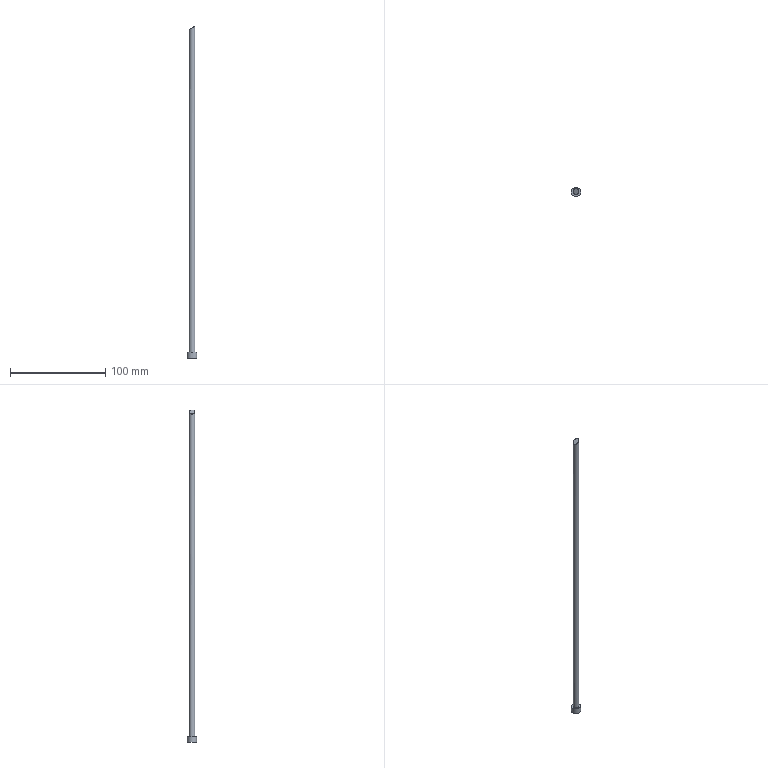Part | NX | features solid 2 | 1 solid | 5 faces | box 10 x 10 x 349.469 mm | volume 10125 mm3 | cylinder 2 | plane 2 | spline 1 | commonest cylinder face diameters 6 x1 10 x1
STEP:
#1=CARTESIAN_POINT('',(-26.5,31.,-339.5));
#2=VERTEX_POINT('',#1);
#3=CARTESIAN_POINT('',(-29.5,31.,-339.5));
#4=DIRECTION('',(0.,0.,-1.));
#5=DIRECTION('',(1.,0.,0.));
#6=AXIS2_PLACEMENT_3D('',#3,#4,#5);
#7=CIRCLE('',#6,3.);
#8=EDGE_CURVE('',#2,#2,#7,.T.);
#9=ORIENTED_EDGE('',*,*,#8,.F.);
#10=EDGE_LOOP('',(#9));
#11=FACE_BOUND('',#10,.T.);
#12=CARTESIAN_POINT('',(-32.484,31.31,-0.2778));
#13=VERTEX_POINT('',#12);
#14=CARTESIAN_POINT('',(-32.419,29.974,-0.1907));
#15=CARTESIAN_POINT('',(-32.583,31.327,-0.3551));
#16=CARTESIAN_POINT('',(-32.152,32.58,-0.05574));
#17=CARTESIAN_POINT('',(-31.061,33.756,0.7394));
#18=CARTESIAN_POINT('',(-29.252,34.244,2.044));
#19=CARTESIAN_POINT('',(-27.478,33.464,3.269));
#20=CARTESIAN_POINT('',(-26.581,32.026,3.891));
#21=CARTESIAN_POINT('',(-26.416,30.688,4.03));
#22=CARTESIAN_POINT('',(-26.845,29.418,3.783));
#23=CARTESIAN_POINT('',(-27.971,28.214,3.068));
#24=CARTESIAN_POINT('',(-29.831,27.764,1.8));
#25=CARTESIAN_POINT('',(-31.544,28.569,0.5156));
#26=CARTESIAN_POINT('',(-32.419,29.974,-0.1907));
#27=CARTESIAN_POINT('',(-32.583,31.327,-0.3551));
#28=CARTESIAN_POINT('',(-32.152,32.58,-0.05574));
#29=B_SPLINE_CURVE_WITH_KNOTS('',3,(#14,#15,#16,#17,#18,#19,#20,#21,#22,#23,#24,#25,#26,#27,#28),.UNSPECIFIED.,.T.,.F.,(1,1,1,1,1,1,1,1,1,1,1,1,1,1,1,1,1,1,1),(-0.005227,-0.002614,-0.001307,0.,0.001307,0.002614,0.005227,0.007841,0.009147,0.01045,0.01176,0.01307,0.01568,0.01829,0.0196,0.02091,0.02222,0.02352,0.02614),.UNSPECIFIED.);
#30=EDGE_CURVE('',#13,#13,#29,.T.);
#31=ORIENTED_EDGE('',*,*,#30,.T.);
#32=EDGE_LOOP('',(#31));
#33=FACE_BOUND('',#32,.T.);
#34=CARTESIAN_POINT('',(-29.5,31.,-345.5));
#35=DIRECTION('',(0.,0.,1.));
#36=DIRECTION('',(1.,0.,0.));
#37=AXIS2_PLACEMENT_3D('',#34,#35,#36);
#38=CYLINDRICAL_SURFACE('',#37,3.);
#39=ADVANCED_FACE('',(#11,#33),#38,.T.);
#40=ORIENTED_EDGE('',*,*,#8,.T.);
#41=EDGE_LOOP('',(#40));
#42=FACE_BOUND('',#41,.T.);
#43=CARTESIAN_POINT('',(-24.5,31.,-339.5));
#44=VERTEX_POINT('',#43);
#45=CARTESIAN_POINT('',(-29.5,31.,-339.5));
#46=DIRECTION('',(0.,0.,1.));
#47=DIRECTION('',(1.,0.,0.));
#48=AXIS2_PLACEMENT_3D('',#45,#46,#47);
#49=CIRCLE('',#48,5.);
#50=EDGE_CURVE('',#44,#44,#49,.T.);
#51=ORIENTED_EDGE('',*,*,#50,.T.);
#52=EDGE_LOOP('',(#51));
#53=FACE_BOUND('',#52,.T.);
#54=CARTESIAN_POINT('',(-29.5,31.,-339.5));
#55=DIRECTION('',(0.,0.,1.));
#56=DIRECTION('',(1.,0.,0.));
#57=AXIS2_PLACEMENT_3D('',#54,#55,#56);
#58=PLANE('',#57);
#59=ADVANCED_FACE('',(#42,#53),#58,.T.);
#60=CARTESIAN_POINT('',(-24.5,31.,-345.5));
#61=VERTEX_POINT('',#60);
#62=CARTESIAN_POINT('',(-29.5,31.,-345.5));
#63=DIRECTION('',(0.,0.,-1.));
#64=DIRECTION('',(1.,0.,0.));
#65=AXIS2_PLACEMENT_3D('',#62,#63,#64);
#66=CIRCLE('',#65,5.);
#67=EDGE_CURVE('',#61,#61,#66,.T.);
#68=ORIENTED_EDGE('',*,*,#67,.T.);
#69=EDGE_LOOP('',(#68));
#70=FACE_BOUND('',#69,.T.);
#71=CARTESIAN_POINT('',(-29.5,31.,-345.5));
#72=DIRECTION('',(0.,0.,-1.));
#73=DIRECTION('',(-1.,0.,0.));
#74=AXIS2_PLACEMENT_3D('',#71,#72,#73);
#75=PLANE('',#74);
#76=ADVANCED_FACE('',(#70),#75,.T.);
#77=ORIENTED_EDGE('',*,*,#50,.F.);
#78=EDGE_LOOP('',(#77));
#79=FACE_BOUND('',#78,.T.);
#80=ORIENTED_EDGE('',*,*,#67,.F.);
#81=EDGE_LOOP('',(#80));
#82=FACE_BOUND('',#81,.T.);
#83=CARTESIAN_POINT('',(-29.5,31.,-345.5));
#84=DIRECTION('',(0.,0.,1.));
#85=DIRECTION('',(1.,0.,0.));
#86=AXIS2_PLACEMENT_3D('',#83,#84,#85);
#87=CYLINDRICAL_SURFACE('',#86,5.);
#88=ADVANCED_FACE('',(#79,#82),#87,.T.);
#89=ORIENTED_EDGE('',*,*,#30,.F.);
#90=EDGE_LOOP('',(#89));
#91=FACE_BOUND('',#90,.T.);
#92=CARTESIAN_POINT('',(-32.561,27.941,-0.2468));
#93=CARTESIAN_POINT('',(-32.548,29.98,-0.2906));
#94=CARTESIAN_POINT('',(-32.534,32.019,-0.3353));
#95=CARTESIAN_POINT('',(-32.519,34.059,-0.3807));
#96=CARTESIAN_POINT('',(-30.591,27.941,1.273));
#97=CARTESIAN_POINT('',(-30.579,29.98,1.23));
#98=CARTESIAN_POINT('',(-30.566,32.019,1.186));
#99=CARTESIAN_POINT('',(-30.553,34.059,1.142));
#100=CARTESIAN_POINT('',(-28.557,27.94,2.71));
#101=CARTESIAN_POINT('',(-28.545,29.98,2.669));
#102=CARTESIAN_POINT('',(-28.533,32.019,2.626));
#103=CARTESIAN_POINT('',(-28.52,34.058,2.582));
#104=CARTESIAN_POINT('',(-26.466,27.94,4.063));
#105=CARTESIAN_POINT('',(-26.455,29.979,4.022));
#106=CARTESIAN_POINT('',(-26.444,32.019,3.98));
#107=CARTESIAN_POINT('',(-26.432,34.058,3.938));
#108=B_SPLINE_SURFACE_WITH_KNOTS('',3,3,((#92,#93,#94,#95),(#96,#97,#98,#99),(#100,#101,#102,#103),(#104,#105,#106,#107)),.UNSPECIFIED.,.F.,.F.,.F.,(4,4),(4,4),(0.4606,0.4985),(0.08229,0.1985),.PIECEWISE_BEZIER_KNOTS.);
#109=ADVANCED_FACE('',(#91),#108,.T.);
#110=CLOSED_SHELL('',(#39,#59,#76,#88,#109));
#111=MANIFOLD_SOLID_BREP('',#110);
#112=(LENGTH_UNIT()NAMED_UNIT(*)SI_UNIT(.MILLI.,.METRE.));
#113=UNCERTAINTY_MEASURE_WITH_UNIT(LENGTH_MEASURE(0.0508),#112,'','');
#114=(NAMED_UNIT(*)PLANE_ANGLE_UNIT()SI_UNIT($,.RADIAN.));
#115=(NAMED_UNIT(*)SI_UNIT($,.STERADIAN.)SOLID_ANGLE_UNIT());
#116=(GEOMETRIC_REPRESENTATION_CONTEXT(3)GLOBAL_UNCERTAINTY_ASSIGNED_CONTEXT((#113))GLOBAL_UNIT_ASSIGNED_CONTEXT((#112,#114,#115))REPRESENTATION_CONTEXT('',''));
#117=ADVANCED_BREP_SHAPE_REPRESENTATION('',(#111),#116);